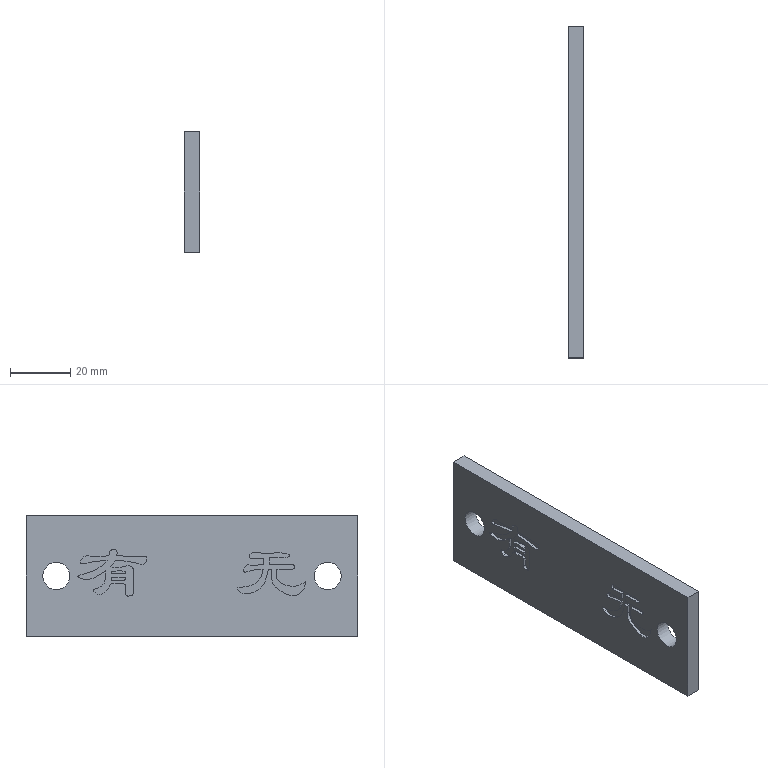Part | NX | features solid 2 | 1 solid | 93 faces | box 5 x 110 x 40 mm | volume 21117 mm3 | spline 68 | plane 23 | cylinder 2 | commonest cylinder face diameters 9 x2